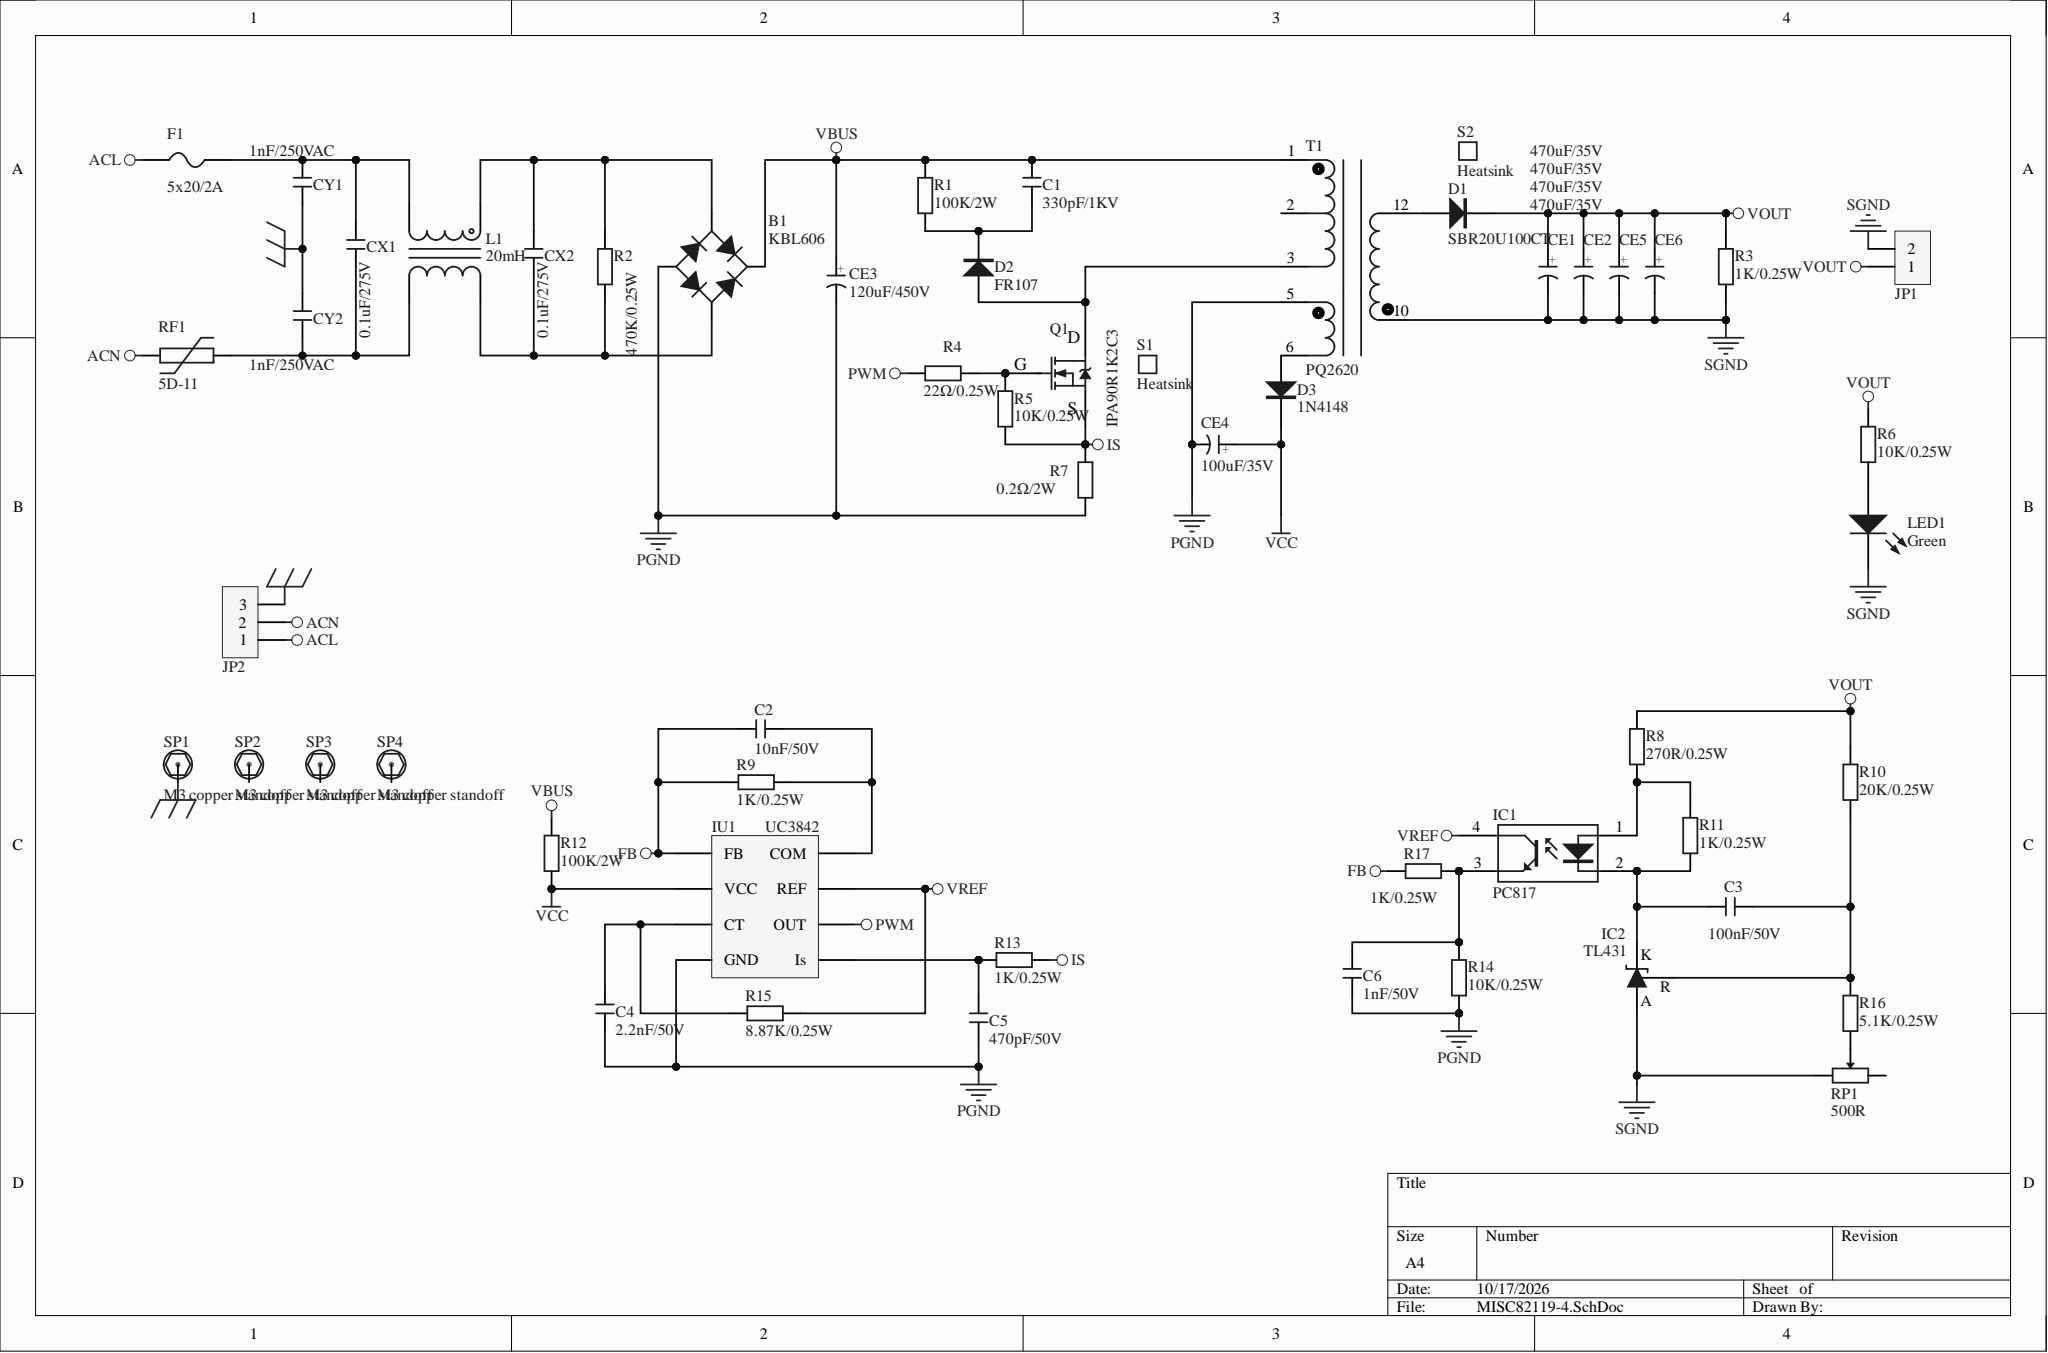Circuit board | Altium Designer | 55 parts | 30 nets
Bill of materials:
Comment,Description,Designator,Footprint,LibRef,Quantity
"KBL606","600V/8A bridge rectifier","B1","KBL","KBL","1"
"330pF/1KV","Ceramic disc capacitor","C1","CY 5*7*2.5","CC","1"
"10nF/50V","Ceramic disc capacitor","C2","CC 2*5","CC","1"
"100nF/50V","Ceramic disc capacitor","C3","CC 2*5","CC","1"
"2.2nF/50V","Ceramic disc capacitor","C4","CC 2*5","CC","1"
"470pF/50V","Ceramic disc capacitor","C5","CC 2*5","CC","1"
"1nF/50V","Ceramic disc capacitor","C6","CC 2*5","CC","1"
"470uF/35V","Through-hole electrolytic capacitor","CE1, CE2, CE5, CE6","CAP 7.5*18*35.5","CE","4"
"120uF/450V","Through-hole electrolytic capacitor","CE3","CAP 7.5*18*35.5","CE","1"
"100uF/35V","Through-hole electrolytic capacitor","CE4","CAP 7.5*18*35.5","CE","1"
"0.1uF/275V","Safety X capacitor","CX1, CX2","CX 10-13*11","CX","2"
"1nF/250VAC","Safety Y capacitor","CY1, CY2","CY 7.5*8*4","CY","2"
"SBR20U100CT","Rectifier diode","D1","TO220A","1N4007","1"
"FR107","Rectifier diode","D2","DO-41","1N4007","1"
"1N4148","Rectifier diode","D3","DO-35","1N4007","1"
"5x20/2A","Through-hole fuse","F1","FU 4x16_V","FU DIP","1"
"PC817","Linear optocoupler","IC1","DIP4-300","817","1"
"TL431","Adjustable precision shunt regulator","IC2","TO92A","TL431-ID","1"
"UC3842","","IU1","DIP8-300","UC3842","1"
"HDR-1X2","2P connector","JP1","KF7620-2P","Header 2","1"
"HDR-1X3","3P connector","JP2","KF7620-3P","Header 3","1"
"20mH","Common-mode choke","L1","UU10.5","L-UU","1"
"Green","Through-hole 3mm LED","LED1","LED 3MM-G","LED-3MM","1"
"IPA90R1K2C3","N-channel MOSFET","Q1","TO220A","IRF840","1"
"100K/2W","Color-band resistor","R1, R12","RS 2W-V6","R-S","2"
"470K/0.25W","Color-band resistor","R2","RS 1/4W","R-S","1"
"1K/0.25W","Color-band resistor","R3, R9, R11, R13, R17","RS 1/4W","R-S","5"
"22Ω/0.25W","Color-band resistor","R4","RS 1/4W","R-S","1"
"10K/0.25W","Color-band resistor","R5, R6, R14","RS 1/4W","R-S","3"
"0.2Ω/2W","Color-band resistor","R7","RS 2W-V6","R-S","1"
"270R/0.25W","Color-band resistor","R8","RS 1/4W","R-S","1"
"20K/0.25W","Color-band resistor","R10","RS 1/4W","R-S","1"
"8.87K/0.25W","Color-band resistor","R15","RS 1/4W","R-S","1"
"5.1K/0.25W","Color-band resistor","R16","RS 1/4W","R-S","1"
"5D-11","PPTC resettable fuse","RF1","TVR-10D","PPTC","1"
"500R","Single-gang potentiometer","RP1","3296W","RP","1"
"Heatsink","Heatsink","S1, S2","SRP16-24-25-P","S1","2"
"M3 copper standoff","Copper standoff","SP1, SP2, SP3, SP4","M3x4+6_N","铜柱加头大焊盘","4"
"PQ2620","12V high-frequency transformer","T1","PQ2625+6PIN","PQ2620","1"
Netlist (Protel format):
[
B1
KBL
KBL606



]
[
C1
CY 5*7*2.5
330pF/1KV



]
[
C2
CC 2*5
10nF/50V



]
[
C3
CC 2*5
100nF/50V



]
[
C4
CC 2*5
2.2nF/50V



]
[
C5
CC 2*5
470pF/50V



]
[
C6
CC 2*5
1nF/50V



]
[
CE1
CAP 7.5*18*35.5
470uF/35V



]
[
CE2
CAP 7.5*18*35.5
470uF/35V



]
[
CE3
CAP 7.5*18*35.5
120uF/450V



]
[
CE4
CAP 7.5*18*35.5
100uF/35V



]
[
CE5
CAP 7.5*18*35.5
470uF/35V



]
[
CE6
CAP 7.5*18*35.5
470uF/35V



]
[
CX1
CX 10-13*11
0.1uF/275V



]
[
CX2
CX 10-13*11
0.1uF/275V



]
[
CY1
CY 7.5*8*4
1nF/250VAC



]
[
CY2
CY 7.5*8*4
1nF/250VAC



]
[
D1
TO220A
SBR20U100CT



]
[
D2
DO-41
FR107



]
[
D3
DO-35
1N4148



]
[
F1
FU 4x16_V
5x20/2A



]
[
IC1
DIP4-300
PC817



]
[
IC2
TO92A
TL431



]
[
IU1
DIP8-300
UC3842



]
[
JP1
KF7620-2P
HDR-1X2



]
[
JP2
KF7620-3P
HDR-1X3



]
[
L1
UU10.5
20mH



]
[
LED1
LED 3MM-G
Green



]
[
Q1
TO220A
IPA90R1K2C3



]
[
R1
RS 2W-V6
100K/2W



]
[
R2
RS 1/4W
470K/0.25W



]
[
R3
RS 1/4W
1K/0.25W



]
[
R4
RS 1/4W
22Ω/0.25W



]
[
R5
RS 1/4W
10K/0.25W



]
[
R6
RS 1/4W
10K/0.25W



]
[
R7
RS 2W-V6
0.2Ω/2W



]
[
R8
RS 1/4W
270R/0.25W



]
[
R9
RS 1/4W
1K/0.25W



]
[
R10
RS 1/4W
20K/0.25W



]
[
R11
RS 1/4W
1K/0.25W



]
[
R12
RS 2W-V6
100K/2W



]
[
R13
RS 1/4W
1K/0.25W



]
[
R14
RS 1/4W
10K/0.25W



]
[
R15
RS 1/4W
8.87K/0.25W



]
[
R16
RS 1/4W
5.1K/0.25W



]
[
R17
RS 1/4W
1K/0.25W



]
[
RF1
TVR-10D
5D-11



]
[
RP1
3296W
500R



]
[
S1
SRP16-24-25-P
Heatsink



]
[
S2
SRP16-24-25-P
Heatsink



]
[
SP1
M3x4+6_N
M3 copper standoff



]
[
SP2
M3x4+6_N
M3 copper standoff



]
[
SP3
M3x4+6_N
M3 copper standoff



]
[
SP4
M3x4+6_N
M3 copper standoff



]
[
T1
PQ2625+6PIN
PQ2620



]
(
VREF
IC1-4
IU1-8
R15-2
)
(
VOUT
CE1-1
CE2-1
CE5-1
CE6-1
D1-2
JP1-1
R3-1
R6-2
R8-1
R10-1
)
(
VCC
CE4-1
D3-2
IU1-7
R12-2
)
(
VBUS
B1-DC+
C1-1
CE3-1
R1-2
R12-1
T1-1
)
(
SGND
CE1-2
CE2-2
CE5-2
CE6-2
IC2-2
JP1-2
LED1-2
R3-2
RP1-1
T1-10
)
(
PWM
IU1-6
R4-2
)
(
PGND
B1-DC-
C4-2
C5-2
C6-1
CE3-2
CE4-2
IU1-5
R7-1
R14-2
T1-5
)
(
PE
CY1-1
CY2-2
JP2-3
SP1-1
)
(
NetR16_2
R16-2
RP1-2
)
(
NetQ1_1
Q1-1
R4-1
R5-2
)
(
NetLED1_1
LED1-1
R6-1
)
(
NetIC1_1
IC1-1
R8-2
R11-1
)
(
NetD3_1
D3-1
T1-6
)
(
NetD2_1
D2-1
Q1-2
T1-3
)
(
NetD1_1
D1-1
T1-12
)
(
NetCX1_2
CX1-2
CY1-2
F1-1
L1-2
)
(
NetCX1_1
CX1-1
CY2-1
L1-3
RF1-2
)
(
NetC6_2
C6-2
IC1-3
R14-1
R17-2
)
(
NetC5_1
C5-1
IU1-3
R13-2
)
(
NetC4_1
C4-1
IU1-4
R15-1
)
(
NetC3_2
C3-2
IC2-1
R10-2
R16-1
)
(
NetC3_1
C3-1
IC1-2
IC2-3
R11-2
)
(
NetC2_2
C2-2
IU1-1
R9-1
)
(
NetC1_2
C1-2
D2-2
R1-1
)
(
NetB1_AC2
B1-AC2
CX2-1
L1-4
R2-2
)
(
NetB1_AC1
B1-AC1
CX2-2
L1-1
R2-1
)
(
IS
Q1-3
R5-1
R7-2
R13-1
)
(
FB
C2-1
IU1-2
R9-2
R17-1
)
(
ACN
JP2-2
RF1-1
)
(
ACL
F1-2
JP2-1
)